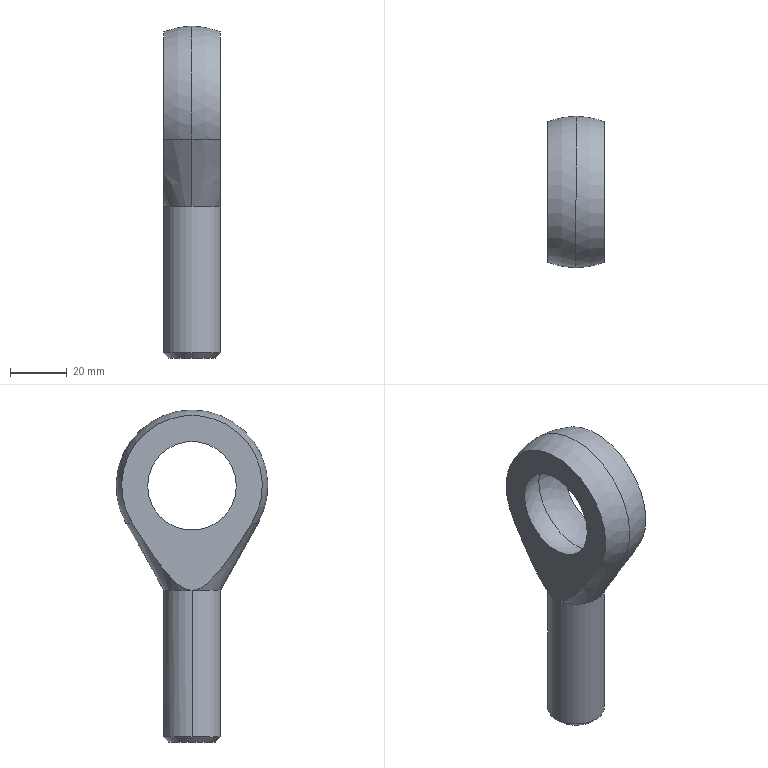Part | STEP file | Electric cylinder end | 1 solid | 14 faces | box 20 x 53.333 x 116.667 mm | volume 46086 mm3 | cone 5 | sphere 4 | plane 3 | cylinder 2 | commonest cylinder face diameters 20 x2
STEP:
#1=CARTESIAN_POINT('',(0.,-10.,235.065));
#2=VERTEX_POINT('',#1);
#3=CARTESIAN_POINT('',(-10.,0.,235.065));
#4=VERTEX_POINT('',#3);
#5=CARTESIAN_POINT('',(0.,0.,235.065));
#6=DIRECTION('',(0.,0.,-1.));
#7=DIRECTION('',(1.,0.,0.));
#8=AXIS2_PLACEMENT_3D('',#5,#6,#7);
#9=CIRCLE('',#8,10.);
#10=EDGE_CURVE('',#2,#4,#9,.T.);
#11=ORIENTED_EDGE('',*,*,#10,.T.);
#12=CARTESIAN_POINT('',(-10.,0.,183.521));
#13=VERTEX_POINT('',#12);
#14=CARTESIAN_POINT('',(-10.,0.,181.732));
#15=DIRECTION('',(0.,0.,-1.));
#16=VECTOR('',#15,1000.);
#17=LINE('',#14,#16);
#18=EDGE_CURVE('',#4,#13,#17,.T.);
#19=ORIENTED_EDGE('',*,*,#18,.T.);
#20=CARTESIAN_POINT('',(0.,-10.,183.521));
#21=VERTEX_POINT('',#20);
#22=CARTESIAN_POINT('',(0.,0.,183.521));
#23=DIRECTION('',(0.,0.,1.));
#24=DIRECTION('',(1.,0.,0.));
#25=AXIS2_PLACEMENT_3D('',#22,#23,#24);
#26=CIRCLE('',#25,10.);
#27=EDGE_CURVE('',#13,#21,#26,.T.);
#28=ORIENTED_EDGE('',*,*,#27,.T.);
#29=CARTESIAN_POINT('',(10.,0.,183.521));
#30=VERTEX_POINT('',#29);
#31=CARTESIAN_POINT('',(0.,0.,183.521));
#32=DIRECTION('',(0.,0.,1.));
#33=DIRECTION('',(1.,0.,0.));
#34=AXIS2_PLACEMENT_3D('',#31,#32,#33);
#35=CIRCLE('',#34,10.);
#36=EDGE_CURVE('',#21,#30,#35,.T.);
#37=ORIENTED_EDGE('',*,*,#36,.T.);
#38=CARTESIAN_POINT('',(10.,0.,235.065));
#39=VERTEX_POINT('',#38);
#40=CARTESIAN_POINT('',(10.,0.,181.732));
#41=DIRECTION('',(0.,0.,-1.));
#42=VECTOR('',#41,1000.);
#43=LINE('',#40,#42);
#44=EDGE_CURVE('',#39,#30,#43,.T.);
#45=ORIENTED_EDGE('',*,*,#44,.F.);
#46=CARTESIAN_POINT('',(0.,0.,235.065));
#47=DIRECTION('',(0.,0.,-1.));
#48=DIRECTION('',(1.,0.,0.));
#49=AXIS2_PLACEMENT_3D('',#46,#47,#48);
#50=CIRCLE('',#49,10.);
#51=EDGE_CURVE('',#39,#2,#50,.T.);
#52=ORIENTED_EDGE('',*,*,#51,.T.);
#53=EDGE_LOOP('',(#11,#19,#28,#37,#45,#52));
#54=FACE_OUTER_BOUND('',#53,.T.);
#55=CARTESIAN_POINT('',(0.,0.,181.732));
#56=DIRECTION('',(0.,0.,-1.));
#57=DIRECTION('',(1.,0.,0.));
#58=AXIS2_PLACEMENT_3D('',#55,#56,#57);
#59=CYLINDRICAL_SURFACE('',#58,10.);
#60=ADVANCED_FACE('',(#54),#59,.T.);
#61=CARTESIAN_POINT('',(0.,-8.211,181.732));
#62=VERTEX_POINT('',#61);
#63=CARTESIAN_POINT('',(0.,8.211,181.732));
#64=VERTEX_POINT('',#63);
#65=CARTESIAN_POINT('',(0.,0.,181.732));
#66=DIRECTION('',(0.,0.,1.));
#67=DIRECTION('',(0.,-1.,0.));
#68=AXIS2_PLACEMENT_3D('',#65,#66,#67);
#69=CIRCLE('',#68,8.211);
#70=EDGE_CURVE('',#62,#64,#69,.T.);
#71=ORIENTED_EDGE('',*,*,#70,.T.);
#72=CARTESIAN_POINT('',(0.,10.,183.521));
#73=VERTEX_POINT('',#72);
#74=CARTESIAN_POINT('',(0.,10.,183.521));
#75=DIRECTION('',(0.,0.7071,0.7071));
#76=VECTOR('',#75,1000.);
#77=LINE('',#74,#76);
#78=EDGE_CURVE('',#64,#73,#77,.T.);
#79=ORIENTED_EDGE('',*,*,#78,.T.);
#80=CARTESIAN_POINT('',(0.,0.,183.521));
#81=DIRECTION('',(0.,0.,1.));
#82=DIRECTION('',(1.,0.,0.));
#83=AXIS2_PLACEMENT_3D('',#80,#81,#82);
#84=CIRCLE('',#83,10.);
#85=EDGE_CURVE('',#30,#73,#84,.T.);
#86=ORIENTED_EDGE('',*,*,#85,.F.);
#87=ORIENTED_EDGE('',*,*,#36,.F.);
#88=CARTESIAN_POINT('',(0.,-10.,183.521));
#89=DIRECTION('',(0.,-0.7071,0.7071));
#90=VECTOR('',#89,1000.);
#91=LINE('',#88,#90);
#92=EDGE_CURVE('',#62,#21,#91,.T.);
#93=ORIENTED_EDGE('',*,*,#92,.F.);
#94=EDGE_LOOP('',(#71,#79,#86,#87,#93));
#95=FACE_OUTER_BOUND('',#94,.T.);
#96=CARTESIAN_POINT('',(0.,0.,183.521));
#97=DIRECTION('',(0.,0.,1.));
#98=DIRECTION('',(0.,-1.,0.));
#99=AXIS2_PLACEMENT_3D('',#96,#97,#98);
#100=CONICAL_SURFACE('',#99,10.,0.7854);
#101=ADVANCED_FACE('',(#95),#100,.T.);
#102=ORIENTED_EDGE('',*,*,#10,.F.);
#103=CARTESIAN_POINT('',(0.,-23.254,258.68));
#104=VERTEX_POINT('',#103);
#105=CARTESIAN_POINT('',(0.,-23.254,258.68));
#106=DIRECTION('',(0.,-0.4894,0.872));
#107=VECTOR('',#106,1000.);
#108=LINE('',#105,#107);
#109=EDGE_CURVE('',#2,#104,#108,.T.);
#110=ORIENTED_EDGE('',*,*,#109,.T.);
#111=CARTESIAN_POINT('',(-10.,-20.994,258.68));
#112=VERTEX_POINT('',#111);
#113=CARTESIAN_POINT('',(0.,0.,258.68));
#114=DIRECTION('',(0.,0.,-1.));
#115=DIRECTION('',(1.,0.,0.));
#116=AXIS2_PLACEMENT_3D('',#113,#114,#115);
#117=CIRCLE('',#116,23.254);
#118=EDGE_CURVE('',#104,#112,#117,.T.);
#119=ORIENTED_EDGE('',*,*,#118,.T.);
#120=CARTESIAN_POINT('',(-10.,-20.994,258.68));
#121=CARTESIAN_POINT('',(-10.,-19.568,256.386));
#122=CARTESIAN_POINT('',(-10.,-18.123,254.103));
#123=CARTESIAN_POINT('',(-10.,-15.904,250.713));
#124=CARTESIAN_POINT('',(-10.,-15.155,249.589));
#125=CARTESIAN_POINT('',(-10.,-13.63,247.358));
#126=CARTESIAN_POINT('',(-10.,-12.855,246.252));
#127=CARTESIAN_POINT('',(-10.,-11.264,244.069));
#128=CARTESIAN_POINT('',(-10.,-10.448,242.992));
#129=CARTESIAN_POINT('',(-10.,-8.746,240.893));
#130=CARTESIAN_POINT('',(-10.,-7.865,239.873));
#131=CARTESIAN_POINT('',(-10.,-6.447,238.436));
#132=CARTESIAN_POINT('',(-10.,-5.958,237.972));
#133=CARTESIAN_POINT('',(-10.,-4.928,237.095));
#134=CARTESIAN_POINT('',(-10.,-4.385,236.68));
#135=CARTESIAN_POINT('',(-10.,-3.529,236.136));
#136=CARTESIAN_POINT('',(-10.,-3.236,235.968));
#137=CARTESIAN_POINT('',(-10.,-2.63,235.664));
#138=CARTESIAN_POINT('',(-10.,-2.315,235.528));
#139=CARTESIAN_POINT('',(-10.,-1.676,235.305));
#140=CARTESIAN_POINT('',(-10.,-1.35,235.217));
#141=CARTESIAN_POINT('',(-10.,-0.6846,235.097));
#142=CARTESIAN_POINT('',(-10.,-0.3424,235.065));
#143=CARTESIAN_POINT('',(-10.,0.,235.065));
#144=B_SPLINE_CURVE_WITH_KNOTS('',3,(#120,#121,#122,#123,#124,#125,#126,#127,#128,#129,#130,#131,#132,#133,#134,#135,#136,#137,#138,#139,#140,#141,#142,#143),.UNSPECIFIED.,.F.,.F.,(4,2,2,2,2,2,2,2,2,2,2,4),(0.,0.008104,0.01216,0.01621,0.02026,0.02431,0.02634,0.02836,0.02938,0.03039,0.0314,0.03242),.UNSPECIFIED.);
#145=EDGE_CURVE('',#112,#4,#144,.T.);
#146=ORIENTED_EDGE('',*,*,#145,.T.);
#147=EDGE_LOOP('',(#102,#110,#119,#146));
#148=FACE_OUTER_BOUND('',#147,.T.);
#149=CARTESIAN_POINT('',(0.,0.,258.68));
#150=DIRECTION('',(0.,0.,1.));
#151=DIRECTION('',(0.,-1.,0.));
#152=AXIS2_PLACEMENT_3D('',#149,#150,#151);
#153=CONICAL_SURFACE('',#152,23.254,0.5115);
#154=ADVANCED_FACE('',(#148),#153,.T.);
#155=CARTESIAN_POINT('',(0.,23.254,258.68));
#156=VERTEX_POINT('',#155);
#157=CARTESIAN_POINT('',(10.,20.994,258.68));
#158=VERTEX_POINT('',#157);
#159=CARTESIAN_POINT('',(0.,0.,258.68));
#160=DIRECTION('',(0.,0.,-1.));
#161=DIRECTION('',(0.,-1.,0.));
#162=AXIS2_PLACEMENT_3D('',#159,#160,#161);
#163=CIRCLE('',#162,23.254);
#164=EDGE_CURVE('',#156,#158,#163,.T.);
#165=ORIENTED_EDGE('',*,*,#164,.F.);
#166=CARTESIAN_POINT('',(0.,0.,298.399));
#167=VERTEX_POINT('',#166);
#168=CARTESIAN_POINT('',(0.,0.,271.732));
#169=DIRECTION('',(1.,0.,0.));
#170=DIRECTION('',(0.,1.,0.));
#171=AXIS2_PLACEMENT_3D('',#168,#169,#170);
#172=CIRCLE('',#171,26.667);
#173=EDGE_CURVE('',#156,#167,#172,.T.);
#174=ORIENTED_EDGE('',*,*,#173,.T.);
#175=CARTESIAN_POINT('',(0.,0.,271.732));
#176=DIRECTION('',(-1.,0.,0.));
#177=DIRECTION('',(0.,-1.,0.));
#178=AXIS2_PLACEMENT_3D('',#175,#176,#177);
#179=CIRCLE('',#178,26.667);
#180=EDGE_CURVE('',#104,#167,#179,.T.);
#181=ORIENTED_EDGE('',*,*,#180,.F.);
#182=CARTESIAN_POINT('',(10.,-20.994,258.68));
#183=VERTEX_POINT('',#182);
#184=CARTESIAN_POINT('',(0.,0.,258.68));
#185=DIRECTION('',(0.,0.,-1.));
#186=DIRECTION('',(1.,0.,0.));
#187=AXIS2_PLACEMENT_3D('',#184,#185,#186);
#188=CIRCLE('',#187,23.254);
#189=EDGE_CURVE('',#183,#104,#188,.T.);
#190=ORIENTED_EDGE('',*,*,#189,.F.);
#191=CARTESIAN_POINT('',(10.,0.,271.732));
#192=DIRECTION('',(-1.,0.,0.));
#193=DIRECTION('',(0.,-1.,0.));
#194=AXIS2_PLACEMENT_3D('',#191,#192,#193);
#195=CIRCLE('',#194,24.721);
#196=EDGE_CURVE('',#183,#158,#195,.T.);
#197=ORIENTED_EDGE('',*,*,#196,.T.);
#198=EDGE_LOOP('',(#165,#174,#181,#190,#197));
#199=FACE_OUTER_BOUND('',#198,.T.);
#200=CARTESIAN_POINT('',(0.,0.,271.732));
#201=DIRECTION('',(1.,0.,0.));
#202=DIRECTION('',(0.,-1.,0.));
#203=AXIS2_PLACEMENT_3D('',#200,#201,#202);
#204=SPHERICAL_SURFACE('',#203,26.667);
#205=ADVANCED_FACE('',(#199),#204,.T.);
#206=CARTESIAN_POINT('',(10.,-15.594,271.732));
#207=VERTEX_POINT('',#206);
#208=CARTESIAN_POINT('',(10.,15.594,271.732));
#209=VERTEX_POINT('',#208);
#210=CARTESIAN_POINT('',(10.,0.,271.732));
#211=DIRECTION('',(-1.,0.,0.));
#212=DIRECTION('',(0.,-1.,0.));
#213=AXIS2_PLACEMENT_3D('',#210,#211,#212);
#214=CIRCLE('',#213,15.594);
#215=EDGE_CURVE('',#207,#209,#214,.T.);
#216=ORIENTED_EDGE('',*,*,#215,.F.);
#217=CARTESIAN_POINT('',(10.,0.,271.732));
#218=DIRECTION('',(-1.,0.,0.));
#219=DIRECTION('',(0.,-1.,0.));
#220=AXIS2_PLACEMENT_3D('',#217,#218,#219);
#221=CIRCLE('',#220,15.594);
#222=EDGE_CURVE('',#209,#207,#221,.T.);
#223=ORIENTED_EDGE('',*,*,#222,.F.);
#224=EDGE_LOOP('',(#216,#223));
#225=FACE_BOUND('',#224,.T.);
#226=CARTESIAN_POINT('',(0.,0.,253.207));
#227=VERTEX_POINT('',#226);
#228=CARTESIAN_POINT('',(0.,0.,290.257));
#229=VERTEX_POINT('',#228);
#230=CARTESIAN_POINT('',(0.,0.,271.732));
#231=DIRECTION('',(1.,0.,0.));
#232=DIRECTION('',(0.,1.,0.));
#233=AXIS2_PLACEMENT_3D('',#230,#231,#232);
#234=CIRCLE('',#233,18.525);
#235=EDGE_CURVE('',#227,#229,#234,.T.);
#236=ORIENTED_EDGE('',*,*,#235,.F.);
#237=CARTESIAN_POINT('',(0.,0.,271.732));
#238=DIRECTION('',(-1.,0.,0.));
#239=DIRECTION('',(0.,-1.,0.));
#240=AXIS2_PLACEMENT_3D('',#237,#238,#239);
#241=CIRCLE('',#240,18.525);
#242=EDGE_CURVE('',#227,#229,#241,.T.);
#243=ORIENTED_EDGE('',*,*,#242,.T.);
#244=EDGE_LOOP('',(#236,#243));
#245=FACE_OUTER_BOUND('',#244,.T.);
#246=CARTESIAN_POINT('',(0.,0.,271.732));
#247=DIRECTION('',(-1.,0.,0.));
#248=DIRECTION('',(0.,1.,0.));
#249=AXIS2_PLACEMENT_3D('',#246,#247,#248);
#250=SPHERICAL_SURFACE('',#249,18.525);
#251=ADVANCED_FACE('',(#225,#245),#250,.F.);
#252=ORIENTED_EDGE('',*,*,#18,.F.);
#253=CARTESIAN_POINT('',(0.,0.,235.065));
#254=DIRECTION('',(0.,0.,-1.));
#255=DIRECTION('',(1.,0.,0.));
#256=AXIS2_PLACEMENT_3D('',#253,#254,#255);
#257=CIRCLE('',#256,10.);
#258=EDGE_CURVE('',#4,#39,#257,.T.);
#259=ORIENTED_EDGE('',*,*,#258,.T.);
#260=ORIENTED_EDGE('',*,*,#44,.T.);
#261=ORIENTED_EDGE('',*,*,#85,.T.);
#262=CARTESIAN_POINT('',(0.,0.,183.521));
#263=DIRECTION('',(0.,0.,1.));
#264=DIRECTION('',(1.,0.,0.));
#265=AXIS2_PLACEMENT_3D('',#262,#263,#264);
#266=CIRCLE('',#265,10.);
#267=EDGE_CURVE('',#73,#13,#266,.T.);
#268=ORIENTED_EDGE('',*,*,#267,.T.);
#269=EDGE_LOOP('',(#252,#259,#260,#261,#268));
#270=FACE_OUTER_BOUND('',#269,.T.);
#271=CARTESIAN_POINT('',(0.,0.,181.732));
#272=DIRECTION('',(0.,0.,-1.));
#273=DIRECTION('',(1.,0.,0.));
#274=AXIS2_PLACEMENT_3D('',#271,#272,#273);
#275=CYLINDRICAL_SURFACE('',#274,10.);
#276=ADVANCED_FACE('',(#270),#275,.T.);
#277=ORIENTED_EDGE('',*,*,#78,.F.);
#278=CARTESIAN_POINT('',(0.,0.,181.732));
#279=DIRECTION('',(0.,0.,1.));
#280=DIRECTION('',(0.,-1.,0.));
#281=AXIS2_PLACEMENT_3D('',#278,#279,#280);
#282=CIRCLE('',#281,8.211);
#283=EDGE_CURVE('',#64,#62,#282,.T.);
#284=ORIENTED_EDGE('',*,*,#283,.T.);
#285=ORIENTED_EDGE('',*,*,#92,.T.);
#286=ORIENTED_EDGE('',*,*,#27,.F.);
#287=ORIENTED_EDGE('',*,*,#267,.F.);
#288=EDGE_LOOP('',(#277,#284,#285,#286,#287));
#289=FACE_OUTER_BOUND('',#288,.T.);
#290=CARTESIAN_POINT('',(0.,0.,183.521));
#291=DIRECTION('',(0.,0.,1.));
#292=DIRECTION('',(0.,-1.,0.));
#293=AXIS2_PLACEMENT_3D('',#290,#291,#292);
#294=CONICAL_SURFACE('',#293,10.,0.7854);
#295=ADVANCED_FACE('',(#289),#294,.T.);
#296=ORIENTED_EDGE('',*,*,#109,.F.);
#297=ORIENTED_EDGE('',*,*,#51,.F.);
#298=CARTESIAN_POINT('',(10.,0.,235.065));
#299=CARTESIAN_POINT('',(10.,-0.6916,235.065));
#300=CARTESIAN_POINT('',(10.,-1.358,235.193));
#301=CARTESIAN_POINT('',(10.,-2.328,235.533));
#302=CARTESIAN_POINT('',(10.,-2.645,235.671));
#303=CARTESIAN_POINT('',(10.,-3.253,235.977));
#304=CARTESIAN_POINT('',(10.,-3.547,236.147));
#305=CARTESIAN_POINT('',(10.,-4.12,236.512));
#306=CARTESIAN_POINT('',(10.,-4.399,236.708));
#307=CARTESIAN_POINT('',(10.,-4.944,237.119));
#308=CARTESIAN_POINT('',(10.,-5.211,237.335));
#309=CARTESIAN_POINT('',(10.,-5.987,237.999));
#310=CARTESIAN_POINT('',(10.,-6.477,238.465));
#311=CARTESIAN_POINT('',(10.,-7.895,239.906));
#312=CARTESIAN_POINT('',(10.,-8.772,240.924));
#313=CARTESIAN_POINT('',(10.,-10.464,243.014));
#314=CARTESIAN_POINT('',(10.,-11.276,244.086));
#315=CARTESIAN_POINT('',(10.,-12.864,246.264));
#316=CARTESIAN_POINT('',(10.,-13.638,247.369));
#317=CARTESIAN_POINT('',(10.,-15.161,249.598));
#318=CARTESIAN_POINT('',(10.,-15.909,250.721));
#319=CARTESIAN_POINT('',(10.,-18.126,254.107));
#320=CARTESIAN_POINT('',(10.,-19.569,256.388));
#321=CARTESIAN_POINT('',(10.,-20.994,258.68));
#322=B_SPLINE_CURVE_WITH_KNOTS('',3,(#298,#299,#300,#301,#302,#303,#304,#305,#306,#307,#308,#309,#310,#311,#312,#313,#314,#315,#316,#317,#318,#319,#320,#321),.UNSPECIFIED.,.F.,.F.,(4,2,2,2,2,2,2,2,2,2,2,4),(0.,0.002035,0.003053,0.00407,0.005088,0.006106,0.008141,0.01221,0.01628,0.02035,0.02442,0.03256),.UNSPECIFIED.);
#323=EDGE_CURVE('',#39,#183,#322,.T.);
#324=ORIENTED_EDGE('',*,*,#323,.T.);
#325=ORIENTED_EDGE('',*,*,#189,.T.);
#326=EDGE_LOOP('',(#296,#297,#324,#325));
#327=FACE_OUTER_BOUND('',#326,.T.);
#328=CARTESIAN_POINT('',(0.,0.,258.68));
#329=DIRECTION('',(0.,0.,1.));
#330=DIRECTION('',(0.,-1.,0.));
#331=AXIS2_PLACEMENT_3D('',#328,#329,#330);
#332=CONICAL_SURFACE('',#331,23.254,0.5115);
#333=ADVANCED_FACE('',(#327),#332,.T.);
#334=ORIENTED_EDGE('',*,*,#70,.F.);
#335=ORIENTED_EDGE('',*,*,#283,.F.);
#336=EDGE_LOOP('',(#334,#335));
#337=FACE_OUTER_BOUND('',#336,.T.);
#338=CARTESIAN_POINT('',(-8.211,0.,181.732));
#339=DIRECTION('',(0.,0.,1.));
#340=DIRECTION('',(-1.,0.,0.));
#341=AXIS2_PLACEMENT_3D('',#338,#339,#340);
#342=PLANE('',#341);
#343=ADVANCED_FACE('',(#337),#342,.F.);
#344=CARTESIAN_POINT('',(10.,20.994,258.68));
#345=CARTESIAN_POINT('',(10.,19.568,256.386));
#346=CARTESIAN_POINT('',(10.,18.123,254.103));
#347=CARTESIAN_POINT('',(10.,15.904,250.713));
#348=CARTESIAN_POINT('',(10.,15.155,249.589));
#349=CARTESIAN_POINT('',(10.,13.63,247.358));
#350=CARTESIAN_POINT('',(10.,12.855,246.252));
#351=CARTESIAN_POINT('',(10.,11.264,244.069));
#352=CARTESIAN_POINT('',(10.,10.448,242.992));
#353=CARTESIAN_POINT('',(10.,8.746,240.893));
#354=CARTESIAN_POINT('',(10.,7.865,239.873));
#355=CARTESIAN_POINT('',(10.,6.447,238.436));
#356=CARTESIAN_POINT('',(10.,5.958,237.972));
#357=CARTESIAN_POINT('',(10.,4.928,237.095));
#358=CARTESIAN_POINT('',(10.,4.385,236.68));
#359=CARTESIAN_POINT('',(10.,3.529,236.136));
#360=CARTESIAN_POINT('',(10.,3.236,235.968));
#361=CARTESIAN_POINT('',(10.,2.63,235.664));
#362=CARTESIAN_POINT('',(10.,2.315,235.528));
#363=CARTESIAN_POINT('',(10.,1.676,235.305));
#364=CARTESIAN_POINT('',(10.,1.35,235.217));
#365=CARTESIAN_POINT('',(10.,0.6846,235.097));
#366=CARTESIAN_POINT('',(10.,0.3424,235.065));
#367=CARTESIAN_POINT('',(10.,0.,235.065));
#368=B_SPLINE_CURVE_WITH_KNOTS('',3,(#344,#345,#346,#347,#348,#349,#350,#351,#352,#353,#354,#355,#356,#357,#358,#359,#360,#361,#362,#363,#364,#365,#366,#367),.UNSPECIFIED.,.F.,.F.,(4,2,2,2,2,2,2,2,2,2,2,4),(0.,0.008104,0.01216,0.01621,0.02026,0.02431,0.02634,0.02836,0.02938,0.03039,0.0314,0.03242),.UNSPECIFIED.);
#369=EDGE_CURVE('',#158,#39,#368,.T.);
#370=ORIENTED_EDGE('',*,*,#369,.T.);
#371=ORIENTED_EDGE('',*,*,#258,.F.);
#372=CARTESIAN_POINT('',(-10.,20.994,258.68));
#373=VERTEX_POINT('',#372);
#374=CARTESIAN_POINT('',(-10.,0.,235.065));
#375=CARTESIAN_POINT('',(-10.,0.6916,235.065));
#376=CARTESIAN_POINT('',(-10.,1.358,235.193));
#377=CARTESIAN_POINT('',(-10.,2.328,235.533));
#378=CARTESIAN_POINT('',(-10.,2.645,235.671));
#379=CARTESIAN_POINT('',(-10.,3.253,235.977));
#380=CARTESIAN_POINT('',(-10.,3.547,236.147));
#381=CARTESIAN_POINT('',(-10.,4.12,236.512));
#382=CARTESIAN_POINT('',(-10.,4.399,236.708));
#383=CARTESIAN_POINT('',(-10.,4.944,237.119));
#384=CARTESIAN_POINT('',(-10.,5.211,237.335));
#385=CARTESIAN_POINT('',(-10.,5.987,237.999));
#386=CARTESIAN_POINT('',(-10.,6.477,238.465));
#387=CARTESIAN_POINT('',(-10.,7.895,239.906));
#388=CARTESIAN_POINT('',(-10.,8.772,240.924));
#389=CARTESIAN_POINT('',(-10.,10.464,243.014));
#390=CARTESIAN_POINT('',(-10.,11.276,244.086));
#391=CARTESIAN_POINT('',(-10.,12.864,246.264));
#392=CARTESIAN_POINT('',(-10.,13.638,247.369));
#393=CARTESIAN_POINT('',(-10.,15.161,249.598));
#394=CARTESIAN_POINT('',(-10.,15.909,250.721));
#395=CARTESIAN_POINT('',(-10.,18.126,254.107));
#396=CARTESIAN_POINT('',(-10.,19.569,256.388));
#397=CARTESIAN_POINT('',(-10.,20.994,258.68));
#398=B_SPLINE_CURVE_WITH_KNOTS('',3,(#374,#375,#376,#377,#378,#379,#380,#381,#382,#383,#384,#385,#386,#387,#388,#389,#390,#391,#392,#393,#394,#395,#396,#397),.UNSPECIFIED.,.F.,.F.,(4,2,2,2,2,2,2,2,2,2,2,4),(0.,0.002035,0.003053,0.00407,0.005088,0.006106,0.008141,0.01221,0.01628,0.02035,0.02442,0.03256),.UNSPECIFIED.);
#399=EDGE_CURVE('',#4,#373,#398,.T.);
#400=ORIENTED_EDGE('',*,*,#399,.T.);
#401=CARTESIAN_POINT('',(0.,0.,258.68));
#402=DIRECTION('',(0.,0.,-1.));
#403=DIRECTION('',(0.,-1.,0.));
#404=AXIS2_PLACEMENT_3D('',#401,#402,#403);
#405=CIRCLE('',#404,23.254);
#406=EDGE_CURVE('',#373,#156,#405,.T.);
#407=ORIENTED_EDGE('',*,*,#406,.T.);
#408=ORIENTED_EDGE('',*,*,#164,.T.);
#409=EDGE_LOOP('',(#370,#371,#400,#407,#408));
#410=FACE_OUTER_BOUND('',#409,.T.);
#411=CARTESIAN_POINT('',(0.,0.,258.68));
#412=DIRECTION('',(0.,0.,1.));
#413=DIRECTION('',(0.,-1.,0.));
#414=AXIS2_PLACEMENT_3D('',#411,#412,#413);
#415=CONICAL_SURFACE('',#414,23.254,0.5115);
#416=ADVANCED_FACE('',(#410),#415,.T.);
#417=ORIENTED_EDGE('',*,*,#173,.F.);
#418=ORIENTED_EDGE('',*,*,#406,.F.);
#419=CARTESIAN_POINT('',(-10.,0.,271.732));
#420=DIRECTION('',(1.,0.,0.));
#421=DIRECTION('',(0.,1.,0.));
#422=AXIS2_PLACEMENT_3D('',#419,#420,#421);
#423=CIRCLE('',#422,24.721);
#424=EDGE_CURVE('',#373,#112,#423,.T.);
#425=ORIENTED_EDGE('',*,*,#424,.T.);
#426=ORIENTED_EDGE('',*,*,#118,.F.);
#427=ORIENTED_EDGE('',*,*,#180,.T.);
#428=EDGE_LOOP('',(#417,#418,#425,#426,#427));
#429=FACE_OUTER_BOUND('',#428,.T.);
#430=CARTESIAN_POINT('',(0.,0.,271.732));
#431=DIRECTION('',(1.,0.,0.));
#432=DIRECTION('',(0.,-1.,0.));
#433=AXIS2_PLACEMENT_3D('',#430,#431,#432);
#434=SPHERICAL_SURFACE('',#433,26.667);
#435=ADVANCED_FACE('',(#429),#434,.T.);
#436=ORIENTED_EDGE('',*,*,#215,.T.);
#437=ORIENTED_EDGE('',*,*,#222,.T.);
#438=EDGE_LOOP('',(#436,#437));
#439=FACE_BOUND('',#438,.T.);
#440=ORIENTED_EDGE('',*,*,#369,.F.);
#441=ORIENTED_EDGE('',*,*,#196,.F.);
#442=ORIENTED_EDGE('',*,*,#323,.F.);
#443=EDGE_LOOP('',(#440,#441,#442));
#444=FACE_OUTER_BOUND('',#443,.T.);
#445=CARTESIAN_POINT('',(10.,0.,296.453));
#446=DIRECTION('',(1.,0.,0.));
#447=DIRECTION('',(0.,-1.,0.));
#448=AXIS2_PLACEMENT_3D('',#445,#446,#447);
#449=PLANE('',#448);
#450=ADVANCED_FACE('',(#439,#444),#449,.T.);
#451=ORIENTED_EDGE('',*,*,#399,.F.);
#452=ORIENTED_EDGE('',*,*,#145,.F.);
#453=ORIENTED_EDGE('',*,*,#424,.F.);
#454=EDGE_LOOP('',(#451,#452,#453));
#455=FACE_OUTER_BOUND('',#454,.T.);
#456=CARTESIAN_POINT('',(-10.,15.594,271.732));
#457=VERTEX_POINT('',#456);
#458=CARTESIAN_POINT('',(-10.,-15.594,271.732));
#459=VERTEX_POINT('',#458);
#460=CARTESIAN_POINT('',(-10.,0.,271.732));
#461=DIRECTION('',(1.,0.,0.));
#462=DIRECTION('',(0.,1.,0.));
#463=AXIS2_PLACEMENT_3D('',#460,#461,#462);
#464=CIRCLE('',#463,15.594);
#465=EDGE_CURVE('',#457,#459,#464,.T.);
#466=ORIENTED_EDGE('',*,*,#465,.T.);
#467=CARTESIAN_POINT('',(-10.,0.,271.732));
#468=DIRECTION('',(1.,0.,0.));
#469=DIRECTION('',(0.,1.,0.));
#470=AXIS2_PLACEMENT_3D('',#467,#468,#469);
#471=CIRCLE('',#470,15.594);
#472=EDGE_CURVE('',#459,#457,#471,.T.);
#473=ORIENTED_EDGE('',*,*,#472,.T.);
#474=EDGE_LOOP('',(#466,#473));
#475=FACE_BOUND('',#474,.T.);
#476=CARTESIAN_POINT('',(-10.,0.,287.326));
#477=DIRECTION('',(-1.,0.,0.));
#478=DIRECTION('',(0.,1.,0.));
#479=AXIS2_PLACEMENT_3D('',#476,#477,#478);
#480=PLANE('',#479);
#481=ADVANCED_FACE('',(#455,#475),#480,.T.);
#482=ORIENTED_EDGE('',*,*,#242,.F.);
#483=ORIENTED_EDGE('',*,*,#235,.T.);
#484=EDGE_LOOP('',(#482,#483));
#485=FACE_OUTER_BOUND('',#484,.T.);
#486=ORIENTED_EDGE('',*,*,#465,.F.);
#487=ORIENTED_EDGE('',*,*,#472,.F.);
#488=EDGE_LOOP('',(#486,#487));
#489=FACE_BOUND('',#488,.T.);
#490=CARTESIAN_POINT('',(0.,0.,271.732));
#491=DIRECTION('',(-1.,0.,0.));
#492=DIRECTION('',(0.,1.,0.));
#493=AXIS2_PLACEMENT_3D('',#490,#491,#492);
#494=SPHERICAL_SURFACE('',#493,18.525);
#495=ADVANCED_FACE('',(#485,#489),#494,.F.);
#496=CLOSED_SHELL('',(#60,#101,#154,#205,#251,#276,#295,#333,#343,#416,#435,#450,#481,#495));
#497=MANIFOLD_SOLID_BREP('',#496);
#498=CARTESIAN_POINT('',(0.,0.,0.));
#499=DIRECTION('',(0.,0.,1.));
#500=DIRECTION('',(1.,0.,0.));
#501=AXIS2_PLACEMENT_3D('',#498,#499,#500);
#502=(LENGTH_UNIT()NAMED_UNIT(*)SI_UNIT(.MILLI.,.METRE.));
#503=UNCERTAINTY_MEASURE_WITH_UNIT(LENGTH_MEASURE(0.00001),#502,'','');
#504=(NAMED_UNIT(*)PLANE_ANGLE_UNIT()SI_UNIT($,.RADIAN.));
#505=(NAMED_UNIT(*)SI_UNIT($,.STERADIAN.)SOLID_ANGLE_UNIT());
#506=(GEOMETRIC_REPRESENTATION_CONTEXT(3)GLOBAL_UNCERTAINTY_ASSIGNED_CONTEXT((#503))GLOBAL_UNIT_ASSIGNED_CONTEXT((#502,#504,#505))REPRESENTATION_CONTEXT('',''));
#507=ADVANCED_BREP_SHAPE_REPRESENTATION('',(#497,#501),#506);